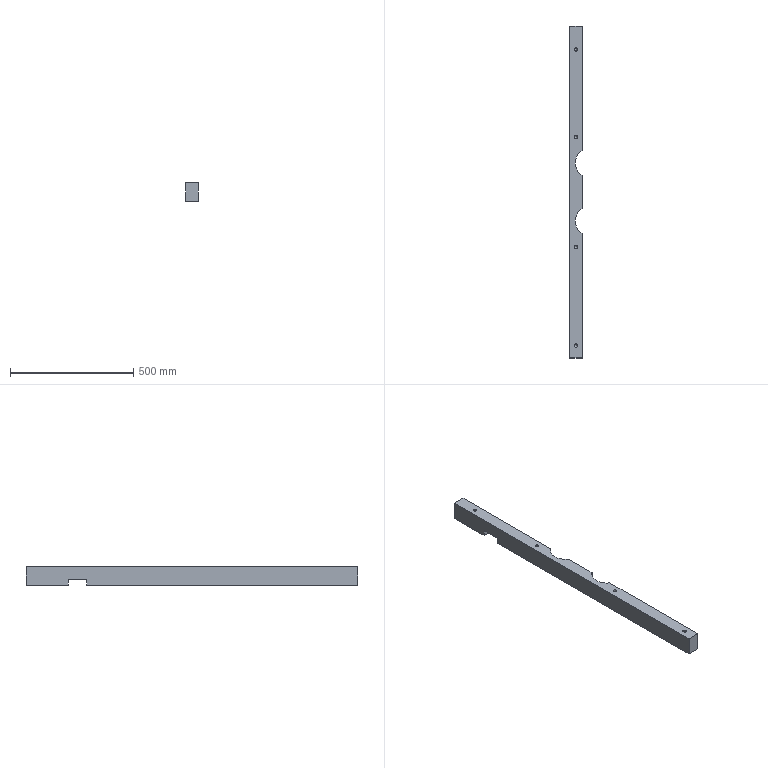Part | NX | features 3 2 | 1 solid | 30 faces | box 50 x 1345 x 75.5 mm | volume 4673845 mm3 | plane 12 | cylinder 10 | cone 8 | commonest cylinder face diameters 14.1 x8 123 x2
STEP:
#1=CARTESIAN_POINT('',(1537.05,222.5,256.5));
#2=VERTEX_POINT('',#1);
#3=CARTESIAN_POINT('',(1530.,222.5,256.5));
#4=DIRECTION('',(0.,0.,-1.));
#5=DIRECTION('',(1.,0.,0.));
#6=AXIS2_PLACEMENT_3D('',#3,#4,#5);
#7=CIRCLE('',#6,7.05);
#8=EDGE_CURVE('',#2,#2,#7,.T.);
#9=ORIENTED_EDGE('',*,*,#8,.T.);
#10=EDGE_LOOP('',(#9));
#11=FACE_BOUND('',#10,.T.);
#12=CARTESIAN_POINT('',(1537.05,-222.5,256.5));
#13=VERTEX_POINT('',#12);
#14=CARTESIAN_POINT('',(1530.,-222.5,256.5));
#15=DIRECTION('',(0.,0.,-1.));
#16=DIRECTION('',(1.,0.,0.));
#17=AXIS2_PLACEMENT_3D('',#14,#15,#16);
#18=CIRCLE('',#17,7.05);
#19=EDGE_CURVE('',#13,#13,#18,.T.);
#20=ORIENTED_EDGE('',*,*,#19,.T.);
#21=EDGE_LOOP('',(#20));
#22=FACE_BOUND('',#21,.T.);
#23=CARTESIAN_POINT('',(1555.,66.753,256.5));
#24=VERTEX_POINT('',#23);
#25=CARTESIAN_POINT('',(1555.,-66.753,256.5));
#26=VERTEX_POINT('',#25);
#27=CARTESIAN_POINT('',(1555.,193.,256.5));
#28=DIRECTION('',(0.,-1.,0.));
#29=VECTOR('',#28,1000.);
#30=LINE('',#27,#29);
#31=EDGE_CURVE('',#24,#26,#30,.T.);
#32=ORIENTED_EDGE('',*,*,#31,.F.);
#33=CARTESIAN_POINT('',(1555.,169.247,256.5));
#34=VERTEX_POINT('',#33);
#35=CARTESIAN_POINT('',(1589.,118.,256.5));
#36=DIRECTION('',(0.,0.,-1.));
#37=DIRECTION('',(1.,0.,0.));
#38=AXIS2_PLACEMENT_3D('',#35,#36,#37);
#39=CIRCLE('',#38,61.5);
#40=EDGE_CURVE('',#24,#34,#39,.T.);
#41=ORIENTED_EDGE('',*,*,#40,.T.);
#42=CARTESIAN_POINT('',(1555.,672.5,256.5));
#43=VERTEX_POINT('',#42);
#44=CARTESIAN_POINT('',(1555.,193.,256.5));
#45=DIRECTION('',(0.,-1.,0.));
#46=VECTOR('',#45,1000.);
#47=LINE('',#44,#46);
#48=EDGE_CURVE('',#43,#34,#47,.T.);
#49=ORIENTED_EDGE('',*,*,#48,.F.);
#50=CARTESIAN_POINT('',(1505.,672.5,256.5));
#51=VERTEX_POINT('',#50);
#52=CARTESIAN_POINT('',(282.5,672.5,256.5));
#53=DIRECTION('',(1.,0.,0.));
#54=VECTOR('',#53,1000.);
#55=LINE('',#52,#54);
#56=EDGE_CURVE('',#51,#43,#55,.T.);
#57=ORIENTED_EDGE('',*,*,#56,.F.);
#58=CARTESIAN_POINT('',(1505.,-672.5,256.5));
#59=VERTEX_POINT('',#58);
#60=CARTESIAN_POINT('',(1505.,193.,256.5));
#61=DIRECTION('',(0.,1.,0.));
#62=VECTOR('',#61,1000.);
#63=LINE('',#60,#62);
#64=EDGE_CURVE('',#59,#51,#63,.T.);
#65=ORIENTED_EDGE('',*,*,#64,.F.);
#66=CARTESIAN_POINT('',(1555.,-672.5,256.5));
#67=VERTEX_POINT('',#66);
#68=CARTESIAN_POINT('',(282.5,-672.5,256.5));
#69=DIRECTION('',(-1.,0.,0.));
#70=VECTOR('',#69,1000.);
#71=LINE('',#68,#70);
#72=EDGE_CURVE('',#67,#59,#71,.T.);
#73=ORIENTED_EDGE('',*,*,#72,.F.);
#74=CARTESIAN_POINT('',(1555.,-169.247,256.5));
#75=VERTEX_POINT('',#74);
#76=CARTESIAN_POINT('',(1555.,193.,256.5));
#77=DIRECTION('',(0.,-1.,0.));
#78=VECTOR('',#77,1000.);
#79=LINE('',#76,#78);
#80=EDGE_CURVE('',#75,#67,#79,.T.);
#81=ORIENTED_EDGE('',*,*,#80,.F.);
#82=CARTESIAN_POINT('',(1589.,-118.,256.5));
#83=DIRECTION('',(0.,0.,1.));
#84=DIRECTION('',(1.,0.,0.));
#85=AXIS2_PLACEMENT_3D('',#82,#83,#84);
#86=CIRCLE('',#85,61.5);
#87=EDGE_CURVE('',#26,#75,#86,.T.);
#88=ORIENTED_EDGE('',*,*,#87,.F.);
#89=EDGE_LOOP('',(#32,#41,#49,#57,#65,#73,#81,#88));
#90=FACE_BOUND('',#89,.T.);
#91=CARTESIAN_POINT('',(1537.05,-622.5,256.5));
#92=VERTEX_POINT('',#91);
#93=CARTESIAN_POINT('',(1530.,-622.5,256.5));
#94=DIRECTION('',(0.,0.,-1.));
#95=DIRECTION('',(1.,0.,0.));
#96=AXIS2_PLACEMENT_3D('',#93,#94,#95);
#97=CIRCLE('',#96,7.05);
#98=EDGE_CURVE('',#92,#92,#97,.T.);
#99=ORIENTED_EDGE('',*,*,#98,.T.);
#100=EDGE_LOOP('',(#99));
#101=FACE_BOUND('',#100,.T.);
#102=CARTESIAN_POINT('',(1537.05,577.5,256.5));
#103=VERTEX_POINT('',#102);
#104=CARTESIAN_POINT('',(1530.,577.5,256.5));
#105=DIRECTION('',(0.,0.,-1.));
#106=DIRECTION('',(1.,0.,0.));
#107=AXIS2_PLACEMENT_3D('',#104,#105,#106);
#108=CIRCLE('',#107,7.05);
#109=EDGE_CURVE('',#103,#103,#108,.T.);
#110=ORIENTED_EDGE('',*,*,#109,.T.);
#111=EDGE_LOOP('',(#110));
#112=FACE_BOUND('',#111,.T.);
#113=CARTESIAN_POINT('',(3545.,0.,256.5));
#114=DIRECTION('',(0.,0.,1.));
#115=DIRECTION('',(-1.,0.,0.));
#116=AXIS2_PLACEMENT_3D('',#113,#114,#115);
#117=PLANE('',#116);
#118=ADVANCED_FACE('',(#11,#22,#90,#101,#112),#117,.T.);
#119=CARTESIAN_POINT('',(1537.05,-622.5,181.));
#120=VERTEX_POINT('',#119);
#121=CARTESIAN_POINT('',(1530.,-622.5,181.));
#122=DIRECTION('',(0.,0.,1.));
#123=DIRECTION('',(1.,0.,0.));
#124=AXIS2_PLACEMENT_3D('',#121,#122,#123);
#125=CIRCLE('',#124,7.05);
#126=EDGE_CURVE('',#120,#120,#125,.T.);
#127=ORIENTED_EDGE('',*,*,#126,.T.);
#128=EDGE_LOOP('',(#127));
#129=FACE_BOUND('',#128,.T.);
#130=CARTESIAN_POINT('',(1555.,426.,181.));
#131=VERTEX_POINT('',#130);
#132=CARTESIAN_POINT('',(1505.,426.,181.));
#133=VERTEX_POINT('',#132);
#134=CARTESIAN_POINT('',(2775.,426.,181.));
#135=DIRECTION('',(-1.,0.,0.));
#136=VECTOR('',#135,1000.);
#137=LINE('',#134,#136);
#138=EDGE_CURVE('',#131,#133,#137,.T.);
#139=ORIENTED_EDGE('',*,*,#138,.F.);
#140=CARTESIAN_POINT('',(1555.,169.247,181.));
#141=VERTEX_POINT('',#140);
#142=CARTESIAN_POINT('',(1555.,193.,181.));
#143=DIRECTION('',(0.,1.,0.));
#144=VECTOR('',#143,1000.);
#145=LINE('',#142,#144);
#146=EDGE_CURVE('',#141,#131,#145,.T.);
#147=ORIENTED_EDGE('',*,*,#146,.F.);
#148=CARTESIAN_POINT('',(1555.,66.753,181.));
#149=VERTEX_POINT('',#148);
#150=CARTESIAN_POINT('',(1589.,118.,181.));
#151=DIRECTION('',(0.,0.,1.));
#152=DIRECTION('',(-1.,0.,0.));
#153=AXIS2_PLACEMENT_3D('',#150,#151,#152);
#154=CIRCLE('',#153,61.5);
#155=EDGE_CURVE('',#141,#149,#154,.T.);
#156=ORIENTED_EDGE('',*,*,#155,.T.);
#157=CARTESIAN_POINT('',(1555.,-66.753,181.));
#158=VERTEX_POINT('',#157);
#159=CARTESIAN_POINT('',(1555.,193.,181.));
#160=DIRECTION('',(0.,1.,0.));
#161=VECTOR('',#160,1000.);
#162=LINE('',#159,#161);
#163=EDGE_CURVE('',#158,#149,#162,.T.);
#164=ORIENTED_EDGE('',*,*,#163,.F.);
#165=CARTESIAN_POINT('',(1555.,-169.247,181.));
#166=VERTEX_POINT('',#165);
#167=CARTESIAN_POINT('',(1589.,-118.,181.));
#168=DIRECTION('',(0.,0.,-1.));
#169=DIRECTION('',(-1.,0.,0.));
#170=AXIS2_PLACEMENT_3D('',#167,#168,#169);
#171=CIRCLE('',#170,61.5);
#172=EDGE_CURVE('',#166,#158,#171,.T.);
#173=ORIENTED_EDGE('',*,*,#172,.F.);
#174=CARTESIAN_POINT('',(1555.,-672.5,181.));
#175=VERTEX_POINT('',#174);
#176=CARTESIAN_POINT('',(1555.,193.,181.));
#177=DIRECTION('',(0.,1.,0.));
#178=VECTOR('',#177,1000.);
#179=LINE('',#176,#178);
#180=EDGE_CURVE('',#175,#166,#179,.T.);
#181=ORIENTED_EDGE('',*,*,#180,.F.);
#182=CARTESIAN_POINT('',(1505.,-672.5,181.));
#183=VERTEX_POINT('',#182);
#184=CARTESIAN_POINT('',(2775.,-672.5,181.));
#185=DIRECTION('',(-1.,0.,0.));
#186=VECTOR('',#185,1000.);
#187=LINE('',#184,#186);
#188=EDGE_CURVE('',#175,#183,#187,.T.);
#189=ORIENTED_EDGE('',*,*,#188,.T.);
#190=CARTESIAN_POINT('',(1505.,193.,181.));
#191=DIRECTION('',(0.,-1.,0.));
#192=VECTOR('',#191,1000.);
#193=LINE('',#190,#192);
#194=EDGE_CURVE('',#133,#183,#193,.T.);
#195=ORIENTED_EDGE('',*,*,#194,.F.);
#196=EDGE_LOOP('',(#139,#147,#156,#164,#173,#181,#189,#195));
#197=FACE_BOUND('',#196,.T.);
#198=CARTESIAN_POINT('',(1537.05,-222.5,181.));
#199=VERTEX_POINT('',#198);
#200=CARTESIAN_POINT('',(1530.,-222.5,181.));
#201=DIRECTION('',(0.,0.,1.));
#202=DIRECTION('',(1.,0.,0.));
#203=AXIS2_PLACEMENT_3D('',#200,#201,#202);
#204=CIRCLE('',#203,7.05);
#205=EDGE_CURVE('',#199,#199,#204,.T.);
#206=ORIENTED_EDGE('',*,*,#205,.T.);
#207=EDGE_LOOP('',(#206));
#208=FACE_BOUND('',#207,.T.);
#209=CARTESIAN_POINT('',(1537.05,222.5,181.));
#210=VERTEX_POINT('',#209);
#211=CARTESIAN_POINT('',(1530.,222.5,181.));
#212=DIRECTION('',(0.,0.,1.));
#213=DIRECTION('',(1.,0.,0.));
#214=AXIS2_PLACEMENT_3D('',#211,#212,#213);
#215=CIRCLE('',#214,7.05);
#216=EDGE_CURVE('',#210,#210,#215,.T.);
#217=ORIENTED_EDGE('',*,*,#216,.T.);
#218=EDGE_LOOP('',(#217));
#219=FACE_BOUND('',#218,.T.);
#220=CARTESIAN_POINT('',(2775.,193.,181.));
#221=DIRECTION('',(0.,0.,-1.));
#222=DIRECTION('',(-1.,0.,0.));
#223=AXIS2_PLACEMENT_3D('',#220,#221,#222);
#224=PLANE('',#223);
#225=ADVANCED_FACE('',(#129,#197,#208,#219),#224,.T.);
#226=CARTESIAN_POINT('',(1505.,502.,181.));
#227=VERTEX_POINT('',#226);
#228=CARTESIAN_POINT('',(1555.,502.,181.));
#229=VERTEX_POINT('',#228);
#230=CARTESIAN_POINT('',(2775.,502.,181.));
#231=DIRECTION('',(1.,0.,0.));
#232=VECTOR('',#231,1000.);
#233=LINE('',#230,#232);
#234=EDGE_CURVE('',#227,#229,#233,.T.);
#235=ORIENTED_EDGE('',*,*,#234,.F.);
#236=CARTESIAN_POINT('',(1505.,672.5,181.));
#237=VERTEX_POINT('',#236);
#238=CARTESIAN_POINT('',(1505.,193.,181.));
#239=DIRECTION('',(0.,-1.,0.));
#240=VECTOR('',#239,1000.);
#241=LINE('',#238,#240);
#242=EDGE_CURVE('',#237,#227,#241,.T.);
#243=ORIENTED_EDGE('',*,*,#242,.F.);
#244=CARTESIAN_POINT('',(1555.,672.5,181.));
#245=VERTEX_POINT('',#244);
#246=CARTESIAN_POINT('',(2775.,672.5,181.));
#247=DIRECTION('',(1.,0.,0.));
#248=VECTOR('',#247,1000.);
#249=LINE('',#246,#248);
#250=EDGE_CURVE('',#237,#245,#249,.T.);
#251=ORIENTED_EDGE('',*,*,#250,.T.);
#252=CARTESIAN_POINT('',(1555.,193.,181.));
#253=DIRECTION('',(0.,1.,0.));
#254=VECTOR('',#253,1000.);
#255=LINE('',#252,#254);
#256=EDGE_CURVE('',#229,#245,#255,.T.);
#257=ORIENTED_EDGE('',*,*,#256,.F.);
#258=EDGE_LOOP('',(#235,#243,#251,#257));
#259=FACE_BOUND('',#258,.T.);
#260=CARTESIAN_POINT('',(1537.05,577.5,181.));
#261=VERTEX_POINT('',#260);
#262=CARTESIAN_POINT('',(1530.,577.5,181.));
#263=DIRECTION('',(0.,0.,1.));
#264=DIRECTION('',(1.,0.,0.));
#265=AXIS2_PLACEMENT_3D('',#262,#263,#264);
#266=CIRCLE('',#265,7.05);
#267=EDGE_CURVE('',#261,#261,#266,.T.);
#268=ORIENTED_EDGE('',*,*,#267,.T.);
#269=EDGE_LOOP('',(#268));
#270=FACE_BOUND('',#269,.T.);
#271=CARTESIAN_POINT('',(2775.,193.,181.));
#272=DIRECTION('',(0.,0.,-1.));
#273=DIRECTION('',(-1.,0.,0.));
#274=AXIS2_PLACEMENT_3D('',#271,#272,#273);
#275=PLANE('',#274);
#276=ADVANCED_FACE('',(#259,#270),#275,.T.);
#277=CARTESIAN_POINT('',(1555.,426.,205.));
#278=VERTEX_POINT('',#277);
#279=CARTESIAN_POINT('',(1555.,426.,-1.5));
#280=DIRECTION('',(0.,0.,-1.));
#281=VECTOR('',#280,1000.);
#282=LINE('',#279,#281);
#283=EDGE_CURVE('',#278,#131,#282,.T.);
#284=ORIENTED_EDGE('',*,*,#283,.F.);
#285=CARTESIAN_POINT('',(1555.,502.,205.));
#286=VERTEX_POINT('',#285);
#287=CARTESIAN_POINT('',(1555.,193.,205.));
#288=DIRECTION('',(0.,-1.,0.));
#289=VECTOR('',#288,1000.);
#290=LINE('',#287,#289);
#291=EDGE_CURVE('',#286,#278,#290,.T.);
#292=ORIENTED_EDGE('',*,*,#291,.F.);
#293=CARTESIAN_POINT('',(1555.,502.,-1.5));
#294=DIRECTION('',(0.,0.,1.));
#295=VECTOR('',#294,1000.);
#296=LINE('',#293,#295);
#297=EDGE_CURVE('',#229,#286,#296,.T.);
#298=ORIENTED_EDGE('',*,*,#297,.F.);
#299=ORIENTED_EDGE('',*,*,#256,.T.);
#300=CARTESIAN_POINT('',(1555.,672.5,-1.5));
#301=DIRECTION('',(0.,0.,1.));
#302=VECTOR('',#301,1000.);
#303=LINE('',#300,#302);
#304=EDGE_CURVE('',#245,#43,#303,.T.);
#305=ORIENTED_EDGE('',*,*,#304,.T.);
#306=ORIENTED_EDGE('',*,*,#48,.T.);
#307=CARTESIAN_POINT('',(1555.,169.247,-181.));
#308=DIRECTION('',(0.,0.,-1.));
#309=VECTOR('',#308,1000.);
#310=LINE('',#307,#309);
#311=EDGE_CURVE('',#34,#141,#310,.T.);
#312=ORIENTED_EDGE('',*,*,#311,.T.);
#313=ORIENTED_EDGE('',*,*,#146,.T.);
#314=EDGE_LOOP('',(#284,#292,#298,#299,#305,#306,#312,#313));
#315=FACE_BOUND('',#314,.T.);
#316=CARTESIAN_POINT('',(1555.,193.,-1.5));
#317=DIRECTION('',(1.,0.,0.));
#318=DIRECTION('',(0.,0.,1.));
#319=AXIS2_PLACEMENT_3D('',#316,#317,#318);
#320=PLANE('',#319);
#321=ADVANCED_FACE('',(#315),#320,.T.);
#322=ORIENTED_EDGE('',*,*,#163,.T.);
#323=CARTESIAN_POINT('',(1555.,66.753,181.));
#324=DIRECTION('',(0.,0.,1.));
#325=VECTOR('',#324,1000.);
#326=LINE('',#323,#325);
#327=EDGE_CURVE('',#149,#24,#326,.T.);
#328=ORIENTED_EDGE('',*,*,#327,.T.);
#329=ORIENTED_EDGE('',*,*,#31,.T.);
#330=CARTESIAN_POINT('',(1555.,-66.753,-181.));
#331=DIRECTION('',(0.,0.,-1.));
#332=VECTOR('',#331,1000.);
#333=LINE('',#330,#332);
#334=EDGE_CURVE('',#26,#158,#333,.T.);
#335=ORIENTED_EDGE('',*,*,#334,.T.);
#336=EDGE_LOOP('',(#322,#328,#329,#335));
#337=FACE_BOUND('',#336,.T.);
#338=CARTESIAN_POINT('',(1555.,193.,-1.5));
#339=DIRECTION('',(1.,0.,0.));
#340=DIRECTION('',(0.,0.,1.));
#341=AXIS2_PLACEMENT_3D('',#338,#339,#340);
#342=PLANE('',#341);
#343=ADVANCED_FACE('',(#337),#342,.T.);
#344=ORIENTED_EDGE('',*,*,#180,.T.);
#345=CARTESIAN_POINT('',(1555.,-169.247,181.));
#346=DIRECTION('',(0.,0.,1.));
#347=VECTOR('',#346,1000.);
#348=LINE('',#345,#347);
#349=EDGE_CURVE('',#166,#75,#348,.T.);
#350=ORIENTED_EDGE('',*,*,#349,.T.);
#351=ORIENTED_EDGE('',*,*,#80,.T.);
#352=CARTESIAN_POINT('',(1555.,-672.5,-1.5));
#353=DIRECTION('',(0.,0.,-1.));
#354=VECTOR('',#353,1000.);
#355=LINE('',#352,#354);
#356=EDGE_CURVE('',#67,#175,#355,.T.);
#357=ORIENTED_EDGE('',*,*,#356,.T.);
#358=EDGE_LOOP('',(#344,#350,#351,#357));
#359=FACE_BOUND('',#358,.T.);
#360=CARTESIAN_POINT('',(1555.,193.,-1.5));
#361=DIRECTION('',(1.,0.,0.));
#362=DIRECTION('',(0.,0.,1.));
#363=AXIS2_PLACEMENT_3D('',#360,#361,#362);
#364=PLANE('',#363);
#365=ADVANCED_FACE('',(#359),#364,.T.);
#366=CARTESIAN_POINT('',(1505.,426.,205.));
#367=VERTEX_POINT('',#366);
#368=CARTESIAN_POINT('',(1505.,426.,-1.5));
#369=DIRECTION('',(0.,0.,1.));
#370=VECTOR('',#369,1000.);
#371=LINE('',#368,#370);
#372=EDGE_CURVE('',#133,#367,#371,.T.);
#373=ORIENTED_EDGE('',*,*,#372,.F.);
#374=ORIENTED_EDGE('',*,*,#194,.T.);
#375=CARTESIAN_POINT('',(1505.,-672.5,-1.5));
#376=DIRECTION('',(0.,0.,1.));
#377=VECTOR('',#376,1000.);
#378=LINE('',#375,#377);
#379=EDGE_CURVE('',#183,#59,#378,.T.);
#380=ORIENTED_EDGE('',*,*,#379,.T.);
#381=ORIENTED_EDGE('',*,*,#64,.T.);
#382=CARTESIAN_POINT('',(1505.,672.5,-1.5));
#383=DIRECTION('',(0.,0.,-1.));
#384=VECTOR('',#383,1000.);
#385=LINE('',#382,#384);
#386=EDGE_CURVE('',#51,#237,#385,.T.);
#387=ORIENTED_EDGE('',*,*,#386,.T.);
#388=ORIENTED_EDGE('',*,*,#242,.T.);
#389=CARTESIAN_POINT('',(1505.,502.,205.));
#390=VERTEX_POINT('',#389);
#391=CARTESIAN_POINT('',(1505.,502.,-1.5));
#392=DIRECTION('',(0.,0.,-1.));
#393=VECTOR('',#392,1000.);
#394=LINE('',#391,#393);
#395=EDGE_CURVE('',#390,#227,#394,.T.);
#396=ORIENTED_EDGE('',*,*,#395,.F.);
#397=CARTESIAN_POINT('',(1505.,193.,205.));
#398=DIRECTION('',(0.,1.,0.));
#399=VECTOR('',#398,1000.);
#400=LINE('',#397,#399);
#401=EDGE_CURVE('',#367,#390,#400,.T.);
#402=ORIENTED_EDGE('',*,*,#401,.F.);
#403=EDGE_LOOP('',(#373,#374,#380,#381,#387,#388,#396,#402));
#404=FACE_BOUND('',#403,.T.);
#405=CARTESIAN_POINT('',(1505.,193.,-1.5));
#406=DIRECTION('',(-1.,0.,0.));
#407=DIRECTION('',(0.,0.,-1.));
#408=AXIS2_PLACEMENT_3D('',#405,#406,#407);
#409=PLANE('',#408);
#410=ADVANCED_FACE('',(#404),#409,.T.);
#411=ORIENTED_EDGE('',*,*,#356,.F.);
#412=ORIENTED_EDGE('',*,*,#72,.T.);
#413=ORIENTED_EDGE('',*,*,#379,.F.);
#414=ORIENTED_EDGE('',*,*,#188,.F.);
#415=EDGE_LOOP('',(#411,#412,#413,#414));
#416=FACE_BOUND('',#415,.T.);
#417=CARTESIAN_POINT('',(282.5,-672.5,-103.));
#418=DIRECTION('',(0.,1.,0.));
#419=DIRECTION('',(1.,0.,0.));
#420=AXIS2_PLACEMENT_3D('',#417,#418,#419);
#421=PLANE('',#420);
#422=ADVANCED_FACE('',(#416),#421,.F.);
#423=ORIENTED_EDGE('',*,*,#386,.F.);
#424=ORIENTED_EDGE('',*,*,#56,.T.);
#425=ORIENTED_EDGE('',*,*,#304,.F.);
#426=ORIENTED_EDGE('',*,*,#250,.F.);
#427=EDGE_LOOP('',(#423,#424,#425,#426));
#428=FACE_BOUND('',#427,.T.);
#429=CARTESIAN_POINT('',(282.5,672.5,101.));
#430=DIRECTION('',(0.,-1.,0.));
#431=DIRECTION('',(-1.,0.,0.));
#432=AXIS2_PLACEMENT_3D('',#429,#430,#431);
#433=PLANE('',#432);
#434=ADVANCED_FACE('',(#428),#433,.F.);
#435=ORIENTED_EDGE('',*,*,#87,.T.);
#436=ORIENTED_EDGE('',*,*,#349,.F.);
#437=ORIENTED_EDGE('',*,*,#172,.T.);
#438=ORIENTED_EDGE('',*,*,#334,.F.);
#439=EDGE_LOOP('',(#435,#436,#437,#438));
#440=FACE_BOUND('',#439,.T.);
#441=CARTESIAN_POINT('',(1589.,-118.,-181.));
#442=DIRECTION('',(0.,0.,1.));
#443=DIRECTION('',(-1.,0.,0.));
#444=AXIS2_PLACEMENT_3D('',#441,#442,#443);
#445=CYLINDRICAL_SURFACE('',#444,61.5);
#446=ADVANCED_FACE('',(#440),#445,.F.);
#447=ORIENTED_EDGE('',*,*,#40,.F.);
#448=ORIENTED_EDGE('',*,*,#327,.F.);
#449=ORIENTED_EDGE('',*,*,#155,.F.);
#450=ORIENTED_EDGE('',*,*,#311,.F.);
#451=EDGE_LOOP('',(#447,#448,#449,#450));
#452=FACE_BOUND('',#451,.T.);
#453=CARTESIAN_POINT('',(1589.,118.,-181.));
#454=DIRECTION('',(0.,0.,1.));
#455=DIRECTION('',(-1.,0.,0.));
#456=AXIS2_PLACEMENT_3D('',#453,#454,#455);
#457=CYLINDRICAL_SURFACE('',#456,61.5);
#458=ADVANCED_FACE('',(#452),#457,.F.);
#459=ORIENTED_EDGE('',*,*,#291,.T.);
#460=CARTESIAN_POINT('',(1510.,426.,205.));
#461=DIRECTION('',(1.,0.,0.));
#462=VECTOR('',#461,1000.);
#463=LINE('',#460,#462);
#464=EDGE_CURVE('',#367,#278,#463,.T.);
#465=ORIENTED_EDGE('',*,*,#464,.F.);
#466=ORIENTED_EDGE('',*,*,#401,.T.);
#467=CARTESIAN_POINT('',(1510.,502.,205.));
#468=DIRECTION('',(-1.,0.,0.));
#469=VECTOR('',#468,1000.);
#470=LINE('',#467,#469);
#471=EDGE_CURVE('',#286,#390,#470,.T.);
#472=ORIENTED_EDGE('',*,*,#471,.F.);
#473=EDGE_LOOP('',(#459,#465,#466,#472));
#474=FACE_BOUND('',#473,.T.);
#475=CARTESIAN_POINT('',(1510.,464.,205.));
#476=DIRECTION('',(0.,0.,1.));
#477=DIRECTION('',(-1.,0.,0.));
#478=AXIS2_PLACEMENT_3D('',#475,#476,#477);
#479=PLANE('',#478);
#480=ADVANCED_FACE('',(#474),#479,.F.);
#481=ORIENTED_EDGE('',*,*,#283,.T.);
#482=ORIENTED_EDGE('',*,*,#138,.T.);
#483=ORIENTED_EDGE('',*,*,#372,.T.);
#484=ORIENTED_EDGE('',*,*,#464,.T.);
#485=EDGE_LOOP('',(#481,#482,#483,#484));
#486=FACE_BOUND('',#485,.T.);
#487=CARTESIAN_POINT('',(1510.,426.,25.));
#488=DIRECTION('',(0.,-1.,0.));
#489=DIRECTION('',(0.,0.,1.));
#490=AXIS2_PLACEMENT_3D('',#487,#488,#489);
#491=PLANE('',#490);
#492=ADVANCED_FACE('',(#486),#491,.F.);
#493=ORIENTED_EDGE('',*,*,#297,.T.);
#494=ORIENTED_EDGE('',*,*,#471,.T.);
#495=ORIENTED_EDGE('',*,*,#395,.T.);
#496=ORIENTED_EDGE('',*,*,#234,.T.);
#497=EDGE_LOOP('',(#493,#494,#495,#496));
#498=FACE_BOUND('',#497,.T.);
#499=CARTESIAN_POINT('',(1510.,502.,25.));
#500=DIRECTION('',(0.,1.,0.));
#501=DIRECTION('',(0.,0.,-1.));
#502=AXIS2_PLACEMENT_3D('',#499,#500,#501);
#503=PLANE('',#502);
#504=ADVANCED_FACE('',(#498),#503,.F.);
#505=CARTESIAN_POINT('',(1537.05,-222.5,188.95));
#506=VERTEX_POINT('',#505);
#507=CARTESIAN_POINT('',(1530.,-222.5,188.95));
#508=DIRECTION('',(0.,0.,1.));
#509=DIRECTION('',(1.,0.,0.));
#510=AXIS2_PLACEMENT_3D('',#507,#508,#509);
#511=CIRCLE('',#510,7.05);
#512=EDGE_CURVE('',#506,#506,#511,.T.);
#513=ORIENTED_EDGE('',*,*,#512,.T.);
#514=EDGE_LOOP('',(#513));
#515=FACE_BOUND('',#514,.T.);
#516=ORIENTED_EDGE('',*,*,#205,.F.);
#517=EDGE_LOOP('',(#516));
#518=FACE_BOUND('',#517,.T.);
#519=CARTESIAN_POINT('',(1530.,-222.5,181.));
#520=DIRECTION('',(0.,0.,1.));
#521=DIRECTION('',(-1.,0.,0.));
#522=AXIS2_PLACEMENT_3D('',#519,#520,#521);
#523=CYLINDRICAL_SURFACE('',#522,7.05);
#524=ADVANCED_FACE('',(#515,#518),#523,.F.);
#525=CARTESIAN_POINT('',(1530.,-222.5,196.));
#526=VERTEX_POINT('',#525);
#527=VERTEX_LOOP('',#526);
#528=FACE_BOUND('',#527,.T.);
#529=ORIENTED_EDGE('',*,*,#512,.F.);
#530=EDGE_LOOP('',(#529));
#531=FACE_BOUND('',#530,.T.);
#532=CARTESIAN_POINT('',(1530.,-222.5,188.95));
#533=DIRECTION('',(0.,0.,-1.));
#534=DIRECTION('',(1.,0.,0.));
#535=AXIS2_PLACEMENT_3D('',#532,#533,#534);
#536=CONICAL_SURFACE('',#535,7.05,0.7854);
#537=ADVANCED_FACE('',(#528,#531),#536,.F.);
#538=CARTESIAN_POINT('',(1537.05,-622.5,188.95));
#539=VERTEX_POINT('',#538);
#540=CARTESIAN_POINT('',(1530.,-622.5,188.95));
#541=DIRECTION('',(0.,0.,1.));
#542=DIRECTION('',(1.,0.,0.));
#543=AXIS2_PLACEMENT_3D('',#540,#541,#542);
#544=CIRCLE('',#543,7.05);
#545=EDGE_CURVE('',#539,#539,#544,.T.);
#546=ORIENTED_EDGE('',*,*,#545,.T.);
#547=EDGE_LOOP('',(#546));
#548=FACE_BOUND('',#547,.T.);
#549=ORIENTED_EDGE('',*,*,#126,.F.);
#550=EDGE_LOOP('',(#549));
#551=FACE_BOUND('',#550,.T.);
#552=CARTESIAN_POINT('',(1530.,-622.5,181.));
#553=DIRECTION('',(0.,0.,1.));
#554=DIRECTION('',(-1.,0.,0.));
#555=AXIS2_PLACEMENT_3D('',#552,#553,#554);
#556=CYLINDRICAL_SURFACE('',#555,7.05);
#557=ADVANCED_FACE('',(#548,#551),#556,.F.);
#558=CARTESIAN_POINT('',(1530.,-622.5,196.));
#559=VERTEX_POINT('',#558);
#560=VERTEX_LOOP('',#559);
#561=FACE_BOUND('',#560,.T.);
#562=ORIENTED_EDGE('',*,*,#545,.F.);
#563=EDGE_LOOP('',(#562));
#564=FACE_BOUND('',#563,.T.);
#565=CARTESIAN_POINT('',(1530.,-622.5,188.95));
#566=DIRECTION('',(0.,0.,-1.));
#567=DIRECTION('',(1.,0.,0.));
#568=AXIS2_PLACEMENT_3D('',#565,#566,#567);
#569=CONICAL_SURFACE('',#568,7.05,0.7854);
#570=ADVANCED_FACE('',(#561,#564),#569,.F.);
#571=CARTESIAN_POINT('',(1537.05,577.5,188.95));
#572=VERTEX_POINT('',#571);
#573=CARTESIAN_POINT('',(1530.,577.5,188.95));
#574=DIRECTION('',(0.,0.,1.));
#575=DIRECTION('',(1.,0.,0.));
#576=AXIS2_PLACEMENT_3D('',#573,#574,#575);
#577=CIRCLE('',#576,7.05);
#578=EDGE_CURVE('',#572,#572,#577,.T.);
#579=ORIENTED_EDGE('',*,*,#578,.T.);
#580=EDGE_LOOP('',(#579));
#581=FACE_BOUND('',#580,.T.);
#582=ORIENTED_EDGE('',*,*,#267,.F.);
#583=EDGE_LOOP('',(#582));
#584=FACE_BOUND('',#583,.T.);
#585=CARTESIAN_POINT('',(1530.,577.5,181.));
#586=DIRECTION('',(0.,0.,1.));
#587=DIRECTION('',(-1.,0.,0.));
#588=AXIS2_PLACEMENT_3D('',#585,#586,#587);
#589=CYLINDRICAL_SURFACE('',#588,7.05);
#590=ADVANCED_FACE('',(#581,#584),#589,.F.);
#591=CARTESIAN_POINT('',(1530.,577.5,196.));
#592=VERTEX_POINT('',#591);
#593=VERTEX_LOOP('',#592);
#594=FACE_BOUND('',#593,.T.);
#595=ORIENTED_EDGE('',*,*,#578,.F.);
#596=EDGE_LOOP('',(#595));
#597=FACE_BOUND('',#596,.T.);
#598=CARTESIAN_POINT('',(1530.,577.5,188.95));
#599=DIRECTION('',(0.,0.,-1.));
#600=DIRECTION('',(1.,0.,0.));
#601=AXIS2_PLACEMENT_3D('',#598,#599,#600);
#602=CONICAL_SURFACE('',#601,7.05,0.7854);
#603=ADVANCED_FACE('',(#594,#597),#602,.F.);
#604=CARTESIAN_POINT('',(1537.05,222.5,188.95));
#605=VERTEX_POINT('',#604);
#606=CARTESIAN_POINT('',(1530.,222.5,188.95));
#607=DIRECTION('',(0.,0.,1.));
#608=DIRECTION('',(1.,0.,0.));
#609=AXIS2_PLACEMENT_3D('',#606,#607,#608);
#610=CIRCLE('',#609,7.05);
#611=EDGE_CURVE('',#605,#605,#610,.T.);
#612=ORIENTED_EDGE('',*,*,#611,.T.);
#613=EDGE_LOOP('',(#612));
#614=FACE_BOUND('',#613,.T.);
#615=ORIENTED_EDGE('',*,*,#216,.F.);
#616=EDGE_LOOP('',(#615));
#617=FACE_BOUND('',#616,.T.);
#618=CARTESIAN_POINT('',(1530.,222.5,181.));
#619=DIRECTION('',(0.,0.,1.));
#620=DIRECTION('',(-1.,0.,0.));
#621=AXIS2_PLACEMENT_3D('',#618,#619,#620);
#622=CYLINDRICAL_SURFACE('',#621,7.05);
#623=ADVANCED_FACE('',(#614,#617),#622,.F.);
#624=CARTESIAN_POINT('',(1530.,222.5,196.));
#625=VERTEX_POINT('',#624);
#626=VERTEX_LOOP('',#625);
#627=FACE_BOUND('',#626,.T.);
#628=ORIENTED_EDGE('',*,*,#611,.F.);
#629=EDGE_LOOP('',(#628));
#630=FACE_BOUND('',#629,.T.);
#631=CARTESIAN_POINT('',(1530.,222.5,188.95));
#632=DIRECTION('',(0.,0.,-1.));
#633=DIRECTION('',(1.,0.,0.));
#634=AXIS2_PLACEMENT_3D('',#631,#632,#633);
#635=CONICAL_SURFACE('',#634,7.05,0.7854);
#636=ADVANCED_FACE('',(#627,#630),#635,.F.);
#637=CARTESIAN_POINT('',(1522.95,-222.5,248.55));
#638=VERTEX_POINT('',#637);
#639=CARTESIAN_POINT('',(1530.,-222.5,248.55));
#640=DIRECTION('',(0.,0.,-1.));
#641=DIRECTION('',(-1.,0.,0.));
#642=AXIS2_PLACEMENT_3D('',#639,#640,#641);
#643=CIRCLE('',#642,7.05);
#644=EDGE_CURVE('',#638,#638,#643,.T.);
#645=ORIENTED_EDGE('',*,*,#644,.T.);
#646=EDGE_LOOP('',(#645));
#647=FACE_BOUND('',#646,.T.);
#648=ORIENTED_EDGE('',*,*,#19,.F.);
#649=EDGE_LOOP('',(#648));
#650=FACE_BOUND('',#649,.T.);
#651=CARTESIAN_POINT('',(1530.,-222.5,256.5));
#652=DIRECTION('',(0.,0.,-1.));
#653=DIRECTION('',(-1.,0.,0.));
#654=AXIS2_PLACEMENT_3D('',#651,#652,#653);
#655=CYLINDRICAL_SURFACE('',#654,7.05);
#656=ADVANCED_FACE('',(#647,#650),#655,.F.);
#657=CARTESIAN_POINT('',(1530.,-222.5,241.5));
#658=VERTEX_POINT('',#657);
#659=VERTEX_LOOP('',#658);
#660=FACE_BOUND('',#659,.T.);
#661=ORIENTED_EDGE('',*,*,#644,.F.);
#662=EDGE_LOOP('',(#661));
#663=FACE_BOUND('',#662,.T.);
#664=CARTESIAN_POINT('',(1530.,-222.5,248.55));
#665=DIRECTION('',(0.,0.,1.));
#666=DIRECTION('',(-1.,0.,0.));
#667=AXIS2_PLACEMENT_3D('',#664,#665,#666);
#668=CONICAL_SURFACE('',#667,7.05,0.7854);
#669=ADVANCED_FACE('',(#660,#663),#668,.F.);
#670=CARTESIAN_POINT('',(1522.95,-622.5,248.55));
#671=VERTEX_POINT('',#670);
#672=CARTESIAN_POINT('',(1530.,-622.5,248.55));
#673=DIRECTION('',(0.,0.,-1.));
#674=DIRECTION('',(-1.,0.,0.));
#675=AXIS2_PLACEMENT_3D('',#672,#673,#674);
#676=CIRCLE('',#675,7.05);
#677=EDGE_CURVE('',#671,#671,#676,.T.);
#678=ORIENTED_EDGE('',*,*,#677,.T.);
#679=EDGE_LOOP('',(#678));
#680=FACE_BOUND('',#679,.T.);
#681=ORIENTED_EDGE('',*,*,#98,.F.);
#682=EDGE_LOOP('',(#681));
#683=FACE_BOUND('',#682,.T.);
#684=CARTESIAN_POINT('',(1530.,-622.5,256.5));
#685=DIRECTION('',(0.,0.,-1.));
#686=DIRECTION('',(-1.,0.,0.));
#687=AXIS2_PLACEMENT_3D('',#684,#685,#686);
#688=CYLINDRICAL_SURFACE('',#687,7.05);
#689=ADVANCED_FACE('',(#680,#683),#688,.F.);
#690=CARTESIAN_POINT('',(1530.,-622.5,241.5));
#691=VERTEX_POINT('',#690);
#692=VERTEX_LOOP('',#691);
#693=FACE_BOUND('',#692,.T.);
#694=ORIENTED_EDGE('',*,*,#677,.F.);
#695=EDGE_LOOP('',(#694));
#696=FACE_BOUND('',#695,.T.);
#697=CARTESIAN_POINT('',(1530.,-622.5,248.55));
#698=DIRECTION('',(0.,0.,1.));
#699=DIRECTION('',(-1.,0.,0.));
#700=AXIS2_PLACEMENT_3D('',#697,#698,#699);
#701=CONICAL_SURFACE('',#700,7.05,0.7854);
#702=ADVANCED_FACE('',(#693,#696),#701,.F.);
#703=CARTESIAN_POINT('',(1522.95,222.5,248.55));
#704=VERTEX_POINT('',#703);
#705=CARTESIAN_POINT('',(1530.,222.5,248.55));
#706=DIRECTION('',(0.,0.,-1.));
#707=DIRECTION('',(-1.,0.,0.));
#708=AXIS2_PLACEMENT_3D('',#705,#706,#707);
#709=CIRCLE('',#708,7.05);
#710=EDGE_CURVE('',#704,#704,#709,.T.);
#711=ORIENTED_EDGE('',*,*,#710,.T.);
#712=EDGE_LOOP('',(#711));
#713=FACE_BOUND('',#712,.T.);
#714=ORIENTED_EDGE('',*,*,#8,.F.);
#715=EDGE_LOOP('',(#714));
#716=FACE_BOUND('',#715,.T.);
#717=CARTESIAN_POINT('',(1530.,222.5,256.5));
#718=DIRECTION('',(0.,0.,-1.));
#719=DIRECTION('',(-1.,0.,0.));
#720=AXIS2_PLACEMENT_3D('',#717,#718,#719);
#721=CYLINDRICAL_SURFACE('',#720,7.05);
#722=ADVANCED_FACE('',(#713,#716),#721,.F.);
#723=CARTESIAN_POINT('',(1530.,222.5,241.5));
#724=VERTEX_POINT('',#723);
#725=VERTEX_LOOP('',#724);
#726=FACE_BOUND('',#725,.T.);
#727=ORIENTED_EDGE('',*,*,#710,.F.);
#728=EDGE_LOOP('',(#727));
#729=FACE_BOUND('',#728,.T.);
#730=CARTESIAN_POINT('',(1530.,222.5,248.55));
#731=DIRECTION('',(0.,0.,1.));
#732=DIRECTION('',(-1.,0.,0.));
#733=AXIS2_PLACEMENT_3D('',#730,#731,#732);
#734=CONICAL_SURFACE('',#733,7.05,0.7854);
#735=ADVANCED_FACE('',(#726,#729),#734,.F.);
#736=CARTESIAN_POINT('',(1522.95,577.5,248.55));
#737=VERTEX_POINT('',#736);
#738=CARTESIAN_POINT('',(1530.,577.5,248.55));
#739=DIRECTION('',(0.,0.,-1.));
#740=DIRECTION('',(-1.,0.,0.));
#741=AXIS2_PLACEMENT_3D('',#738,#739,#740);
#742=CIRCLE('',#741,7.05);
#743=EDGE_CURVE('',#737,#737,#742,.T.);
#744=ORIENTED_EDGE('',*,*,#743,.T.);
#745=EDGE_LOOP('',(#744));
#746=FACE_BOUND('',#745,.T.);
#747=ORIENTED_EDGE('',*,*,#109,.F.);
#748=EDGE_LOOP('',(#747));
#749=FACE_BOUND('',#748,.T.);
#750=CARTESIAN_POINT('',(1530.,577.5,256.5));
#751=DIRECTION('',(0.,0.,-1.));
#752=DIRECTION('',(-1.,0.,0.));
#753=AXIS2_PLACEMENT_3D('',#750,#751,#752);
#754=CYLINDRICAL_SURFACE('',#753,7.05);
#755=ADVANCED_FACE('',(#746,#749),#754,.F.);
#756=CARTESIAN_POINT('',(1530.,577.5,241.5));
#757=VERTEX_POINT('',#756);
#758=VERTEX_LOOP('',#757);
#759=FACE_BOUND('',#758,.T.);
#760=ORIENTED_EDGE('',*,*,#743,.F.);
#761=EDGE_LOOP('',(#760));
#762=FACE_BOUND('',#761,.T.);
#763=CARTESIAN_POINT('',(1530.,577.5,248.55));
#764=DIRECTION('',(0.,0.,1.));
#765=DIRECTION('',(-1.,0.,0.));
#766=AXIS2_PLACEMENT_3D('',#763,#764,#765);
#767=CONICAL_SURFACE('',#766,7.05,0.7854);
#768=ADVANCED_FACE('',(#759,#762),#767,.F.);
#769=CLOSED_SHELL('',(#118,#225,#276,#321,#343,#365,#410,#422,#434,#446,#458,#480,#492,#504,#524,#537,#557,#570,#590,#603,#623,#636,#656,#669,#689,#702,#722,#735,#755,#768));
#770=MANIFOLD_SOLID_BREP('',#769);
#771=(LENGTH_UNIT()NAMED_UNIT(*)SI_UNIT(.MILLI.,.METRE.));
#772=UNCERTAINTY_MEASURE_WITH_UNIT(LENGTH_MEASURE(0.00001),#771,'','');
#773=(NAMED_UNIT(*)PLANE_ANGLE_UNIT()SI_UNIT($,.RADIAN.));
#774=(NAMED_UNIT(*)SI_UNIT($,.STERADIAN.)SOLID_ANGLE_UNIT());
#775=(GEOMETRIC_REPRESENTATION_CONTEXT(3)GLOBAL_UNCERTAINTY_ASSIGNED_CONTEXT((#772))GLOBAL_UNIT_ASSIGNED_CONTEXT((#771,#773,#774))REPRESENTATION_CONTEXT('',''));
#776=ADVANCED_BREP_SHAPE_REPRESENTATION('',(#770),#775);